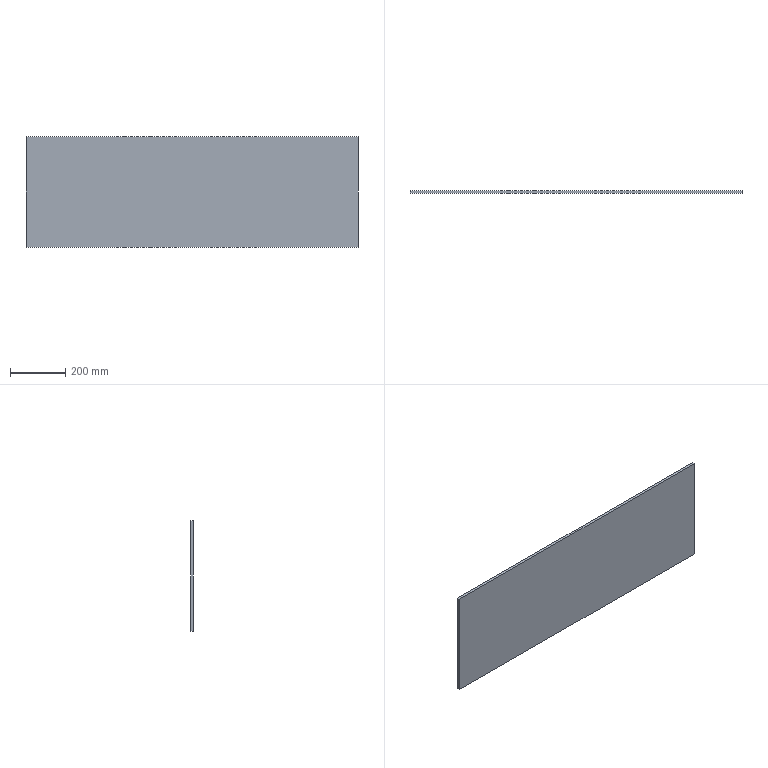Part | SolidWorks | features Extrusion 1 | 1 solid | 6 faces | box 1200 x 10 x 400 mm | volume 4800000 mm3 | plane 6
STEP:
#1=CARTESIAN_POINT('',(600.,0.,200.));
#2=VERTEX_POINT('',#1);
#3=CARTESIAN_POINT('',(600.,0.,-200.));
#4=VERTEX_POINT('',#3);
#5=CARTESIAN_POINT('',(600.,0.,-200.));
#6=DIRECTION('',(0.,0.,-1.));
#7=VECTOR('',#6,1000.);
#8=LINE('',#5,#7);
#9=EDGE_CURVE('',#2,#4,#8,.T.);
#10=ORIENTED_EDGE('',*,*,#9,.T.);
#11=CARTESIAN_POINT('',(600.,10.,-200.));
#12=VERTEX_POINT('',#11);
#13=CARTESIAN_POINT('',(600.,10.,-200.));
#14=DIRECTION('',(0.,-1.,0.));
#15=VECTOR('',#14,1000.);
#16=LINE('',#13,#15);
#17=EDGE_CURVE('',#12,#4,#16,.T.);
#18=ORIENTED_EDGE('',*,*,#17,.F.);
#19=CARTESIAN_POINT('',(600.,10.,200.));
#20=VERTEX_POINT('',#19);
#21=CARTESIAN_POINT('',(600.,10.,-200.));
#22=DIRECTION('',(0.,0.,-1.));
#23=VECTOR('',#22,1000.);
#24=LINE('',#21,#23);
#25=EDGE_CURVE('',#20,#12,#24,.T.);
#26=ORIENTED_EDGE('',*,*,#25,.F.);
#27=CARTESIAN_POINT('',(600.,10.,200.));
#28=DIRECTION('',(0.,-1.,0.));
#29=VECTOR('',#28,1000.);
#30=LINE('',#27,#29);
#31=EDGE_CURVE('',#20,#2,#30,.T.);
#32=ORIENTED_EDGE('',*,*,#31,.T.);
#33=EDGE_LOOP('',(#10,#18,#26,#32));
#34=FACE_OUTER_BOUND('',#33,.T.);
#35=CARTESIAN_POINT('',(600.,10.,-200.));
#36=DIRECTION('',(-1.,0.,0.));
#37=DIRECTION('',(0.,0.,1.));
#38=AXIS2_PLACEMENT_3D('',#35,#36,#37);
#39=PLANE('',#38);
#40=ADVANCED_FACE('',(#34),#39,.F.);
#41=CARTESIAN_POINT('',(-600.,0.,-200.));
#42=VERTEX_POINT('',#41);
#43=CARTESIAN_POINT('',(-600.,0.,-200.));
#44=DIRECTION('',(-1.,0.,0.));
#45=VECTOR('',#44,1000.);
#46=LINE('',#43,#45);
#47=EDGE_CURVE('',#4,#42,#46,.T.);
#48=ORIENTED_EDGE('',*,*,#47,.T.);
#49=CARTESIAN_POINT('',(-600.,10.,-200.));
#50=VERTEX_POINT('',#49);
#51=CARTESIAN_POINT('',(-600.,10.,-200.));
#52=DIRECTION('',(0.,-1.,0.));
#53=VECTOR('',#52,1000.);
#54=LINE('',#51,#53);
#55=EDGE_CURVE('',#50,#42,#54,.T.);
#56=ORIENTED_EDGE('',*,*,#55,.F.);
#57=CARTESIAN_POINT('',(-600.,10.,-200.));
#58=DIRECTION('',(-1.,0.,0.));
#59=VECTOR('',#58,1000.);
#60=LINE('',#57,#59);
#61=EDGE_CURVE('',#12,#50,#60,.T.);
#62=ORIENTED_EDGE('',*,*,#61,.F.);
#63=ORIENTED_EDGE('',*,*,#17,.T.);
#64=EDGE_LOOP('',(#48,#56,#62,#63));
#65=FACE_OUTER_BOUND('',#64,.T.);
#66=CARTESIAN_POINT('',(-600.,10.,-200.));
#67=DIRECTION('',(0.,0.,1.));
#68=DIRECTION('',(1.,0.,0.));
#69=AXIS2_PLACEMENT_3D('',#66,#67,#68);
#70=PLANE('',#69);
#71=ADVANCED_FACE('',(#65),#70,.F.);
#72=CARTESIAN_POINT('',(-600.,0.,200.));
#73=VERTEX_POINT('',#72);
#74=CARTESIAN_POINT('',(-600.,0.,-200.));
#75=DIRECTION('',(0.,0.,1.));
#76=VECTOR('',#75,1000.);
#77=LINE('',#74,#76);
#78=EDGE_CURVE('',#42,#73,#77,.T.);
#79=ORIENTED_EDGE('',*,*,#78,.T.);
#80=CARTESIAN_POINT('',(-600.,10.,200.));
#81=VERTEX_POINT('',#80);
#82=CARTESIAN_POINT('',(-600.,10.,200.));
#83=DIRECTION('',(0.,-1.,0.));
#84=VECTOR('',#83,1000.);
#85=LINE('',#82,#84);
#86=EDGE_CURVE('',#81,#73,#85,.T.);
#87=ORIENTED_EDGE('',*,*,#86,.F.);
#88=CARTESIAN_POINT('',(-600.,10.,-200.));
#89=DIRECTION('',(0.,0.,1.));
#90=VECTOR('',#89,1000.);
#91=LINE('',#88,#90);
#92=EDGE_CURVE('',#50,#81,#91,.T.);
#93=ORIENTED_EDGE('',*,*,#92,.F.);
#94=ORIENTED_EDGE('',*,*,#55,.T.);
#95=EDGE_LOOP('',(#79,#87,#93,#94));
#96=FACE_OUTER_BOUND('',#95,.T.);
#97=CARTESIAN_POINT('',(-600.,10.,-200.));
#98=DIRECTION('',(1.,0.,0.));
#99=DIRECTION('',(0.,0.,-1.));
#100=AXIS2_PLACEMENT_3D('',#97,#98,#99);
#101=PLANE('',#100);
#102=ADVANCED_FACE('',(#96),#101,.F.);
#103=CARTESIAN_POINT('',(-600.,0.,200.));
#104=DIRECTION('',(1.,0.,0.));
#105=VECTOR('',#104,1000.);
#106=LINE('',#103,#105);
#107=EDGE_CURVE('',#73,#2,#106,.T.);
#108=ORIENTED_EDGE('',*,*,#107,.T.);
#109=ORIENTED_EDGE('',*,*,#31,.F.);
#110=CARTESIAN_POINT('',(-600.,10.,200.));
#111=DIRECTION('',(1.,0.,0.));
#112=VECTOR('',#111,1000.);
#113=LINE('',#110,#112);
#114=EDGE_CURVE('',#81,#20,#113,.T.);
#115=ORIENTED_EDGE('',*,*,#114,.F.);
#116=ORIENTED_EDGE('',*,*,#86,.T.);
#117=EDGE_LOOP('',(#108,#109,#115,#116));
#118=FACE_OUTER_BOUND('',#117,.T.);
#119=CARTESIAN_POINT('',(-600.,10.,200.));
#120=DIRECTION('',(0.,0.,-1.));
#121=DIRECTION('',(-1.,0.,0.));
#122=AXIS2_PLACEMENT_3D('',#119,#120,#121);
#123=PLANE('',#122);
#124=ADVANCED_FACE('',(#118),#123,.F.);
#125=ORIENTED_EDGE('',*,*,#25,.T.);
#126=ORIENTED_EDGE('',*,*,#61,.T.);
#127=ORIENTED_EDGE('',*,*,#92,.T.);
#128=ORIENTED_EDGE('',*,*,#114,.T.);
#129=EDGE_LOOP('',(#125,#126,#127,#128));
#130=FACE_OUTER_BOUND('',#129,.T.);
#131=CARTESIAN_POINT('',(0.,10.,0.));
#132=DIRECTION('',(0.,1.,0.));
#133=DIRECTION('',(0.,0.,1.));
#134=AXIS2_PLACEMENT_3D('',#131,#132,#133);
#135=PLANE('',#134);
#136=ADVANCED_FACE('',(#130),#135,.T.);
#137=ORIENTED_EDGE('',*,*,#9,.F.);
#138=ORIENTED_EDGE('',*,*,#107,.F.);
#139=ORIENTED_EDGE('',*,*,#78,.F.);
#140=ORIENTED_EDGE('',*,*,#47,.F.);
#141=EDGE_LOOP('',(#137,#138,#139,#140));
#142=FACE_OUTER_BOUND('',#141,.T.);
#143=CARTESIAN_POINT('',(0.,0.,0.));
#144=DIRECTION('',(0.,1.,0.));
#145=DIRECTION('',(0.,0.,1.));
#146=AXIS2_PLACEMENT_3D('',#143,#144,#145);
#147=PLANE('',#146);
#148=ADVANCED_FACE('',(#142),#147,.F.);
#149=CLOSED_SHELL('',(#40,#71,#102,#124,#136,#148));
#150=MANIFOLD_SOLID_BREP('',#149);
#151=CARTESIAN_POINT('',(0.,0.,0.));
#152=DIRECTION('',(0.,0.,1.));
#153=DIRECTION('',(1.,0.,0.));
#154=AXIS2_PLACEMENT_3D('',#151,#152,#153);
#155=(LENGTH_UNIT()NAMED_UNIT(*)SI_UNIT(.MILLI.,.METRE.));
#156=UNCERTAINTY_MEASURE_WITH_UNIT(LENGTH_MEASURE(0.00001),#155,'','');
#157=(NAMED_UNIT(*)PLANE_ANGLE_UNIT()SI_UNIT($,.RADIAN.));
#158=(NAMED_UNIT(*)SI_UNIT($,.STERADIAN.)SOLID_ANGLE_UNIT());
#159=(GEOMETRIC_REPRESENTATION_CONTEXT(3)GLOBAL_UNCERTAINTY_ASSIGNED_CONTEXT((#156))GLOBAL_UNIT_ASSIGNED_CONTEXT((#155,#157,#158))REPRESENTATION_CONTEXT('',''));
#160=ADVANCED_BREP_SHAPE_REPRESENTATION('',(#150,#154),#159);